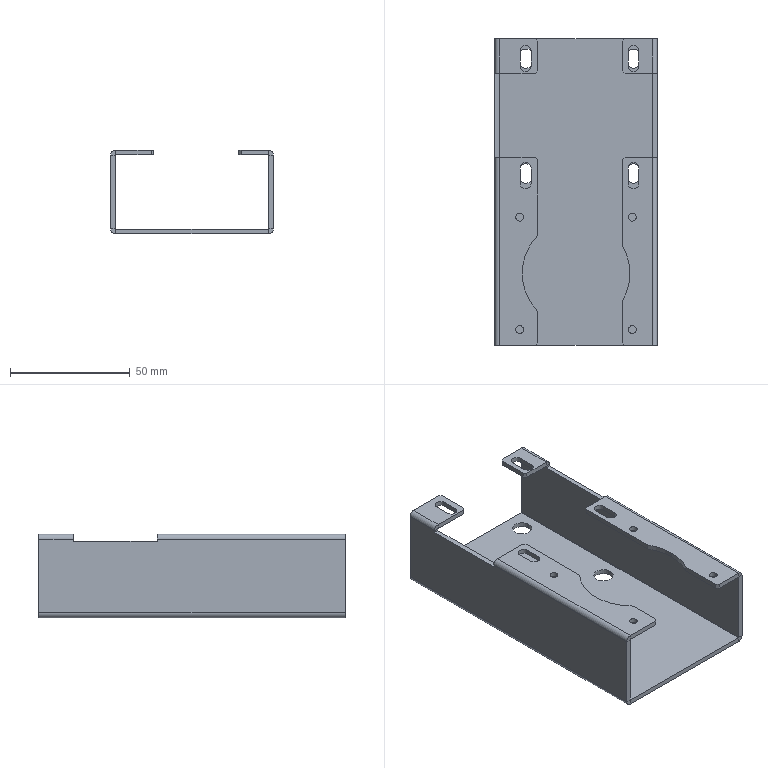Part | STEP file | 1 solid | 107 faces | box 68 x 128 x 35 mm | volume 37554 mm3 | plane 68 | cylinder 39 | commonest cylinder face diameters 3.3 x8 4.5 x8 8 x8 0.2 x6 4.2 x6 45 x3